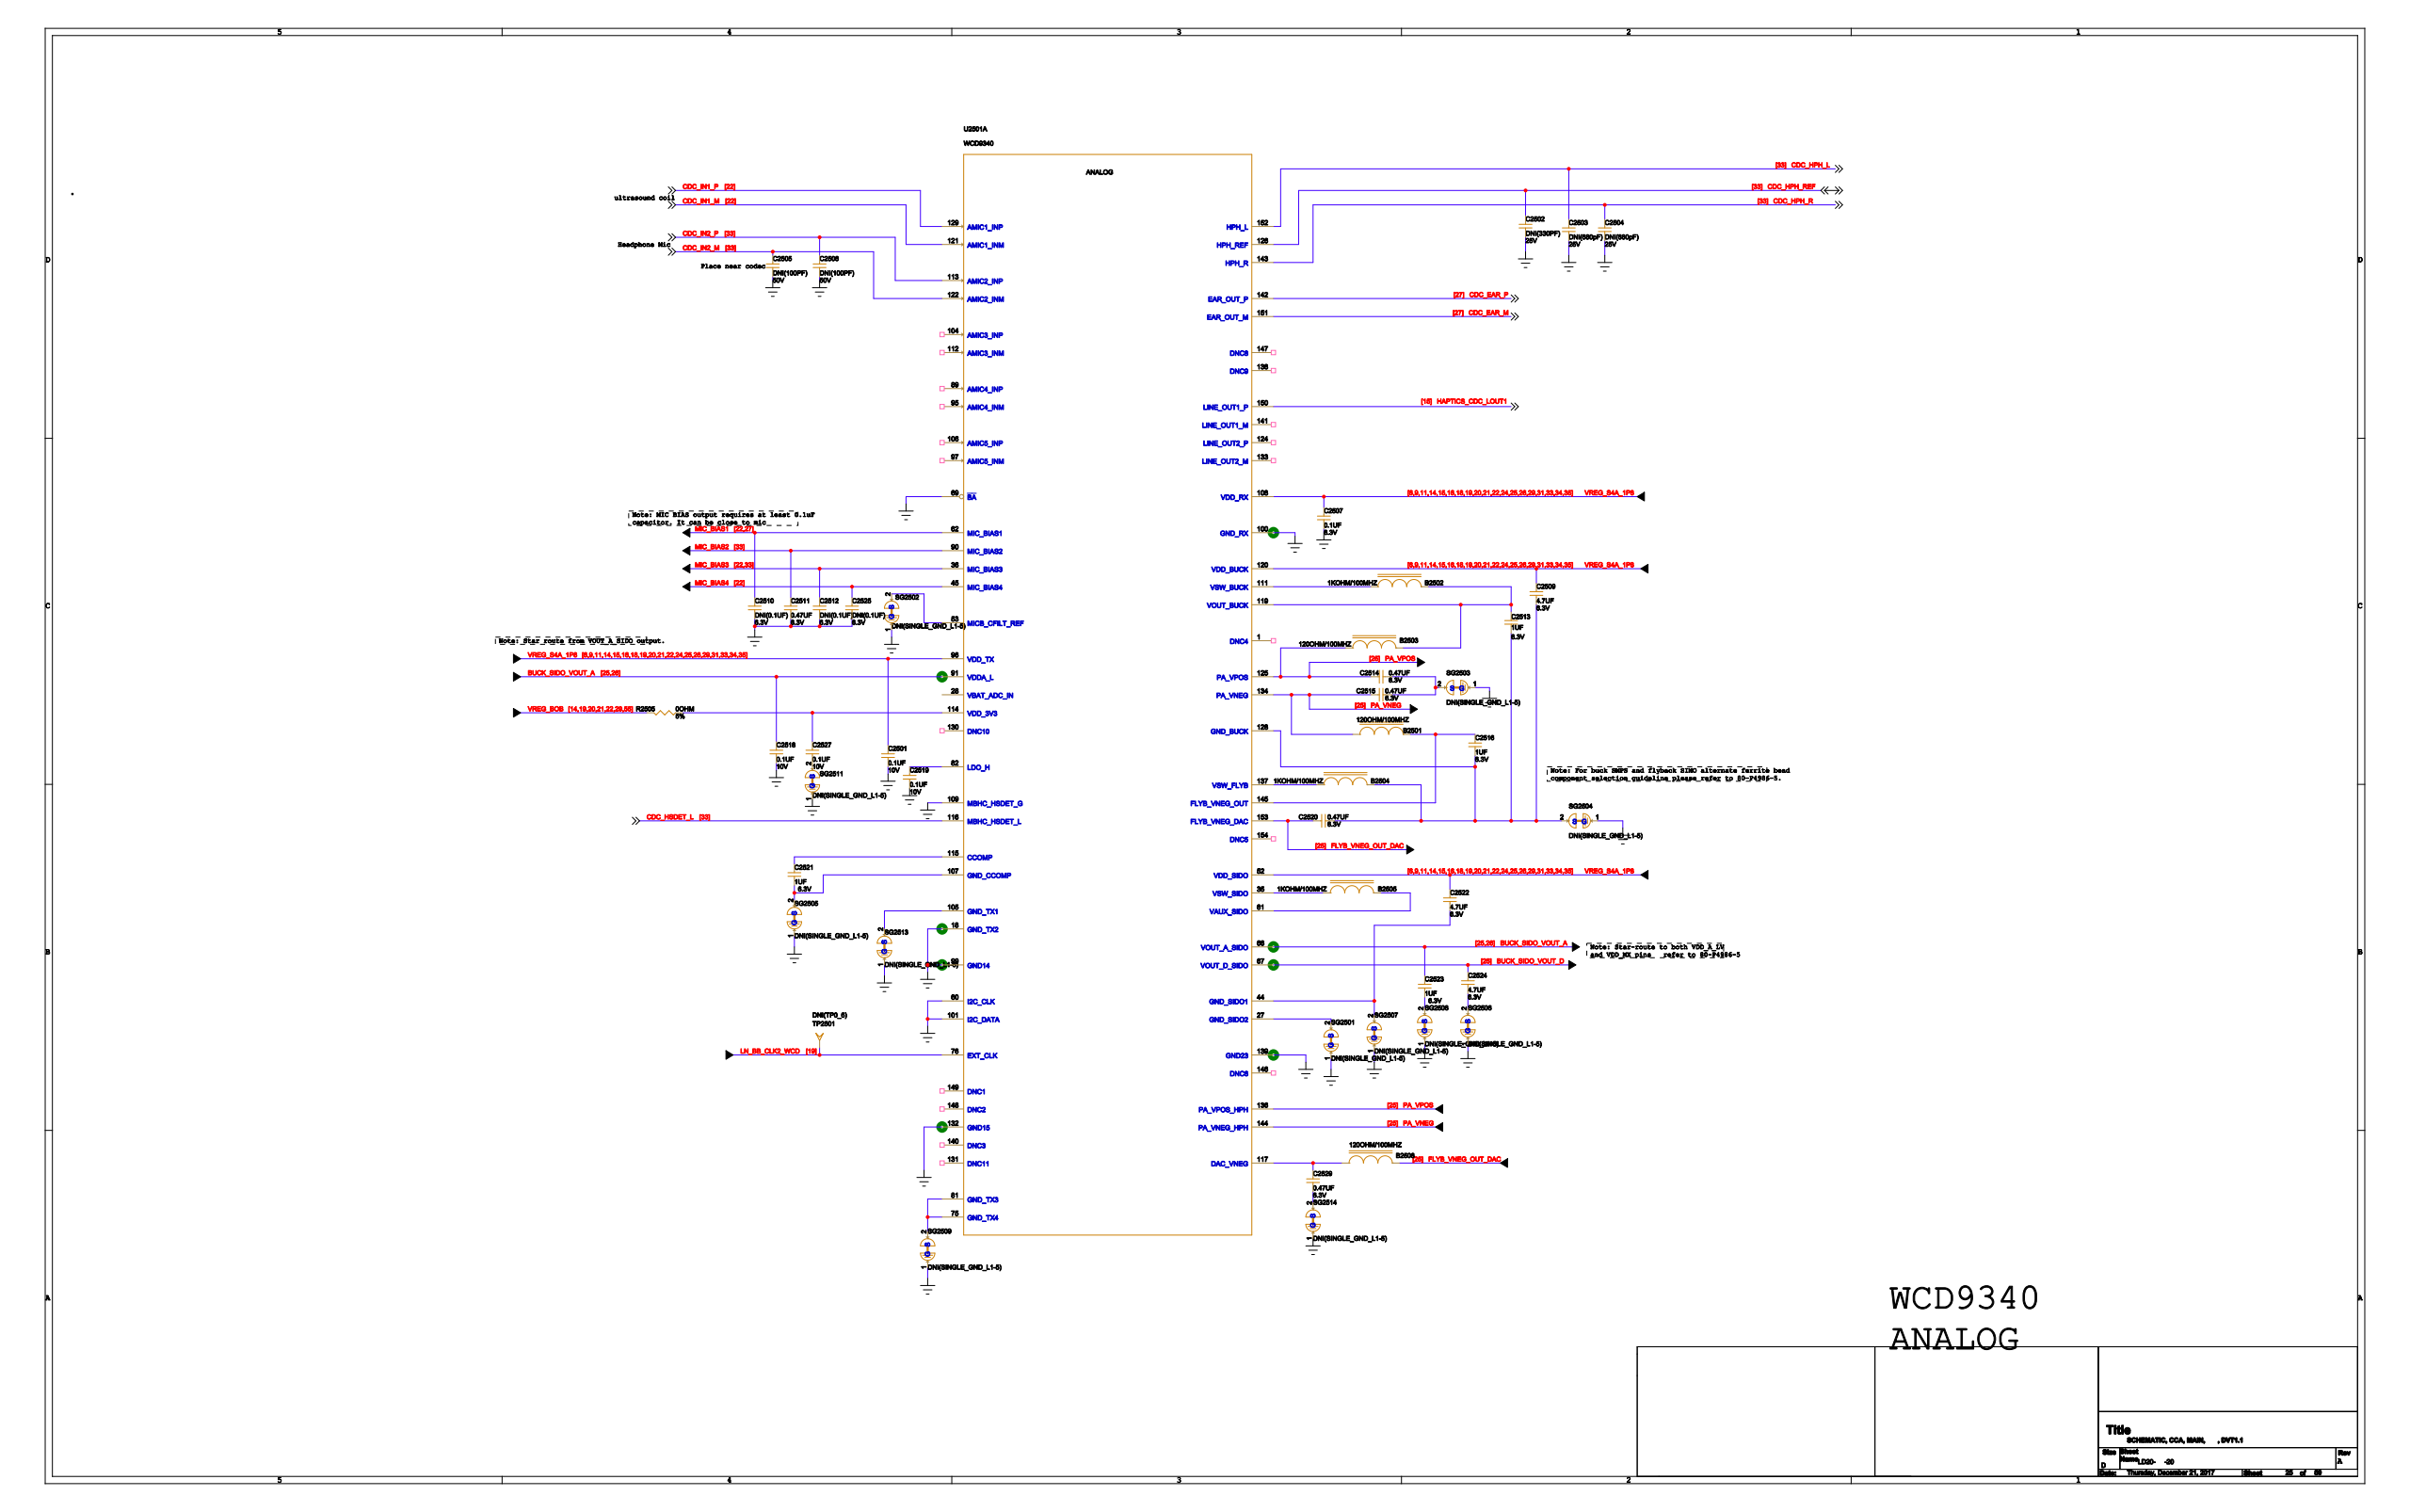Circuit board | Cadence Allegro | 1520 parts | 1149 nets | one sheet of the schematic
Parts on this sheet (reference | value | footprint):
B2501 | 120OHM/100MHZ | 2P0402R
B2502 | 1KOHM/100MHZ | 2P0603R
B2503 | 120OHM/100MHZ | 2P0402R
B2504 | 1KOHM/100MHZ | 2P0603R
B2505 | 1KOHM/100MHZ | 2P0603R
B2508 | 120OHM/100MHZ | 2P0201R
C2501 | 0.1UF | 2P0201R
C2502 | DNI(330PF) | 2P0201R_DNI
C2503 | DNI(680pF) | 2P0201R_DNI
C2504 | DNI(680pF) | 2P0201R_DNI
C2505 | DNI(100PF) | 2P0201R_DNI
C2506 | DNI(100PF) | 2P0201R_DNI
C2507 | 0.1UF | 2P0201R
C2509 | 4.7UF | 2P0402R
C2510 | DNI(0.1uF) | 2P0201R_DNI
C2511 | 0.47UF | 2P0201R
C2512 | DNI(0.1uF) | 2P0201R_DNI
C2513 | 1UF | 2P0201R
C2514 | 0.47UF | 2P0201R
C2515 | 0.47UF | 2P0201R
C2516 | 1UF | 2P0201R
C2518 | 0.1UF | 2P0201R
C2519 | 0.1UF | 2P0201R
C2520 | 0.47UF | 2P0201R
C2521 | 1UF | 2P0201R
C2522 | 4.7UF | 2P0402R
C2523 | 1UF | 2P0201R
C2524 | 4.7UF | 2P0402R
C2525 | DNI(0.1uF) | 2P0201R_DNI
C2527 | 0.1UF | 2P0201R
C2529 | 0.47UF | 2P0201R
R2505 | 0OHM | 2P0201R
SG2501 | DNI(SINGLE_GND_L1-5) | GND_L1-5
SG2502 | DNI(SINGLE_GND_L1-5) | GND_L1-5
SG2503 | DNI(SINGLE_GND_L1-5) | GND_L1-5
SG2504 | DNI(SINGLE_GND_L1-5) | GND_L1-5
SG2505 | DNI(SINGLE_GND_L1-5) | GND_L1-5
SG2506 | DNI(SINGLE_GND_L1-5) | GND_L1-5
SG2507 | DNI(SINGLE_GND_L1-5) | GND_L1-5
SG2508 | DNI(SINGLE_GND_L1-5) | GND_L1-5
SG2509 | DNI(SINGLE_GND_L1-5) | GND_L1-5
SG2511 | DNI(SINGLE_GND_L1-5) | GND_L1-5
SG2513 | DNI(SINGLE_GND_L1-5) | GND_L1-5
SG2514 | DNI(SINGLE_GND_L1-5) | GND_L1-5
TP2501 | DNI(TP0_6) | TP-0_6
U2501 | WCD9340 | 154PGA196X171B138D45
Nets of these parts (net: part-pin ...):
GND: C2501-2 C2502-2 C2503-2 C2504-2 C2505-2 C2506-2 C2507-2 C2510-2 C2511-2 C2512-2 C2518-2 C2519-2 C2525-2 SG2501-1 SG2502-1 SG2503-1 SG2504-1 SG2505-1 SG2506-1 SG2507-1 SG2508-1 SG2509-1 SG2511-1 SG2513-1 SG2514-1 U2501-2 U2501-3 U2501-5 U2501-11 U2501-14 U2501-18 U2501-20 U2501-21 U2501-22 U2501-31 U2501-60 U2501-69 U2501-99 U2501-100 U2501-101 U2501-109 U2501-132 U2501-139
VREG_BOB: R2505-1
VREG_S4A_1P8: C2501-1 C2507-1 C2509-1 C2522-1 U2501-4 U2501-16 U2501-52 U2501-96 U2501-108 U2501-120
N31999226: SG2501-2 U2501-27
N36374127: SG2502-2 U2501-53
N31999373: C2514-2 C2515-2 SG2503-2
N31999335: B2504-2 C2509-2 C2513-2 C2516-2 C2520-2 SG2504-2 U2501-128
N36375294: C2521-2 SG2505-2 U2501-107
N34422743: C2524-2 SG2506-2
N31999271: C2522-2 SG2507-2 U2501-44
N34422914: C2523-2 SG2508-2
N36385849: SG2509-2 U2501-75 U2501-81
N378026801: C2527-2 SG2511-2
N36375460: SG2513-2 U2501-105
N36889559: C2529-2 SG2514-2
MIC_BIAS4: C2525-1 U2501-45
CDC_IN1_P: U2501-129
CDC_IN1_M: U2501-121
MIC_BIAS1: C2510-1 U2501-62
MIC_BIAS3: C2512-1 U2501-36
CDC_IN2_M: C2505-1 U2501-122
CDC_IN2_P: C2506-1 U2501-113
N36375299: C2521-1 U2501-115
N36388958: B2508-1 C2529-1 U2501-117
CDC_EAR_M: U2501-151
CDC_EAR_P: U2501-142
LN_BB_CLK2_WCD: TP2501-1 U2501-76
FLYB_VNEG_OUT_DAC: B2508-2 C2520-1 U2501-153
N31999351: B2501-2 C2516-1 U2501-145
CDC_HPH_L: C2503-1 U2501-152
CDC_HPH_R: C2504-1 U2501-143
CDC_HPH_REF: C2502-1 U2501-126
N36374763: C2519-1 U2501-82
HAPTICS_CDC_LOUT1: U2501-150
CDC_HSDET_L: U2501-116
MIC_BIAS2: C2511-1 U2501-90
PA_VNEG: B2501-1 C2515-1 U2501-134 U2501-144
PA_VPOS: B2503-1 C2514-1 U2501-125 U2501-136
N31999205: B2505-2 U2501-61
VBAT_ADC_IN: U2501-28
BUCK_SIDO_VOUT_A: C2518-1 C2523-1 U2501-19 U2501-26 U2501-68 U2501-91
N36388170: C2527-1 R2505-2 U2501-114
N31999986: B2502-2 B2503-2 C2513-1 U2501-119
BUCK_SIDO_VOUT_D: C2524-1 U2501-67
N31999976: B2502-1 U2501-111
N31999337: B2504-1 U2501-137
N31999209: B2505-1 U2501-35